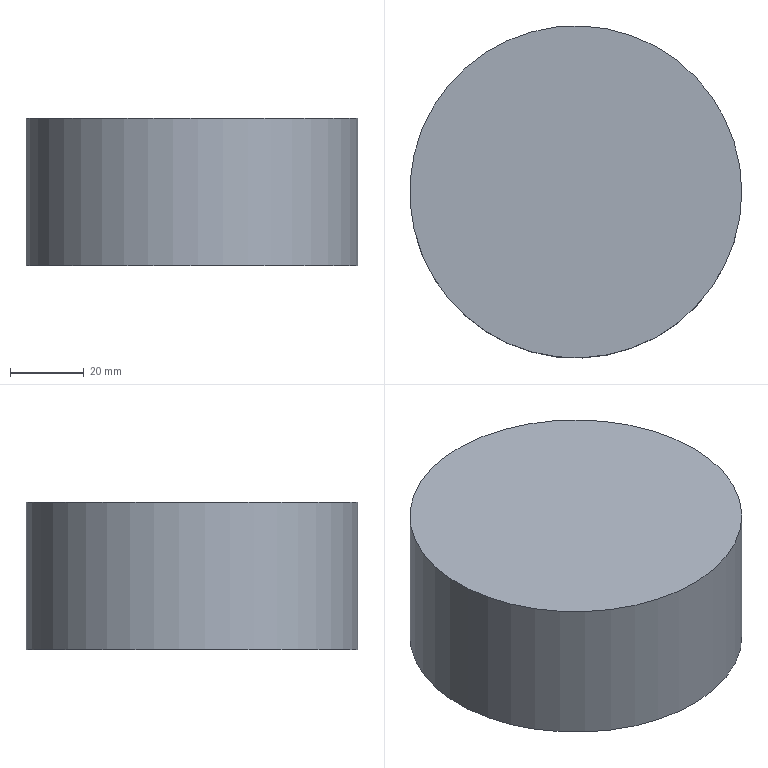Part | NX | features solid 2 | 1 solid | 3 faces | box 90 x 90 x 40 mm | volume 254469 mm3 | plane 2 | cylinder 1 | commonest cylinder face diameters 90 x1
STEP:
#1=CARTESIAN_POINT('',(1245.,-525.,-35.));
#2=VERTEX_POINT('',#1);
#3=CARTESIAN_POINT('',(1200.,-525.,-35.));
#4=DIRECTION('',(0.,0.,1.));
#5=DIRECTION('',(1.,0.,0.));
#6=AXIS2_PLACEMENT_3D('',#3,#4,#5);
#7=CIRCLE('',#6,45.);
#8=EDGE_CURVE('',#2,#2,#7,.T.);
#9=ORIENTED_EDGE('',*,*,#8,.F.);
#10=EDGE_LOOP('',(#9));
#11=FACE_BOUND('',#10,.T.);
#12=CARTESIAN_POINT('',(1245.,-525.,-75.));
#13=VERTEX_POINT('',#12);
#14=CARTESIAN_POINT('',(1200.,-525.,-75.));
#15=DIRECTION('',(0.,0.,1.));
#16=DIRECTION('',(1.,0.,0.));
#17=AXIS2_PLACEMENT_3D('',#14,#15,#16);
#18=CIRCLE('',#17,45.);
#19=EDGE_CURVE('',#13,#13,#18,.T.);
#20=ORIENTED_EDGE('',*,*,#19,.T.);
#21=EDGE_LOOP('',(#20));
#22=FACE_BOUND('',#21,.T.);
#23=CARTESIAN_POINT('',(1200.,-525.,-35.));
#24=DIRECTION('',(0.,0.,-1.));
#25=DIRECTION('',(1.,0.,0.));
#26=AXIS2_PLACEMENT_3D('',#23,#24,#25);
#27=CYLINDRICAL_SURFACE('',#26,45.);
#28=ADVANCED_FACE('',(#11,#22),#27,.T.);
#29=ORIENTED_EDGE('',*,*,#8,.T.);
#30=EDGE_LOOP('',(#29));
#31=FACE_BOUND('',#30,.T.);
#32=CARTESIAN_POINT('',(1200.,-525.,-35.));
#33=DIRECTION('',(0.,0.,-1.));
#34=DIRECTION('',(1.,0.,0.));
#35=AXIS2_PLACEMENT_3D('',#32,#33,#34);
#36=PLANE('',#35);
#37=ADVANCED_FACE('',(#31),#36,.F.);
#38=ORIENTED_EDGE('',*,*,#19,.F.);
#39=EDGE_LOOP('',(#38));
#40=FACE_BOUND('',#39,.T.);
#41=CARTESIAN_POINT('',(1200.,-525.,-75.));
#42=DIRECTION('',(0.,0.,-1.));
#43=DIRECTION('',(1.,0.,0.));
#44=AXIS2_PLACEMENT_3D('',#41,#42,#43);
#45=PLANE('',#44);
#46=ADVANCED_FACE('',(#40),#45,.T.);
#47=CLOSED_SHELL('',(#28,#37,#46));
#48=MANIFOLD_SOLID_BREP('',#47);
#49=(LENGTH_UNIT()NAMED_UNIT(*)SI_UNIT(.MILLI.,.METRE.));
#50=UNCERTAINTY_MEASURE_WITH_UNIT(LENGTH_MEASURE(0.00001),#49,'','');
#51=(NAMED_UNIT(*)PLANE_ANGLE_UNIT()SI_UNIT($,.RADIAN.));
#52=(NAMED_UNIT(*)SI_UNIT($,.STERADIAN.)SOLID_ANGLE_UNIT());
#53=(GEOMETRIC_REPRESENTATION_CONTEXT(3)GLOBAL_UNCERTAINTY_ASSIGNED_CONTEXT((#50))GLOBAL_UNIT_ASSIGNED_CONTEXT((#49,#51,#52))REPRESENTATION_CONTEXT('',''));
#54=ADVANCED_BREP_SHAPE_REPRESENTATION('',(#48),#53);